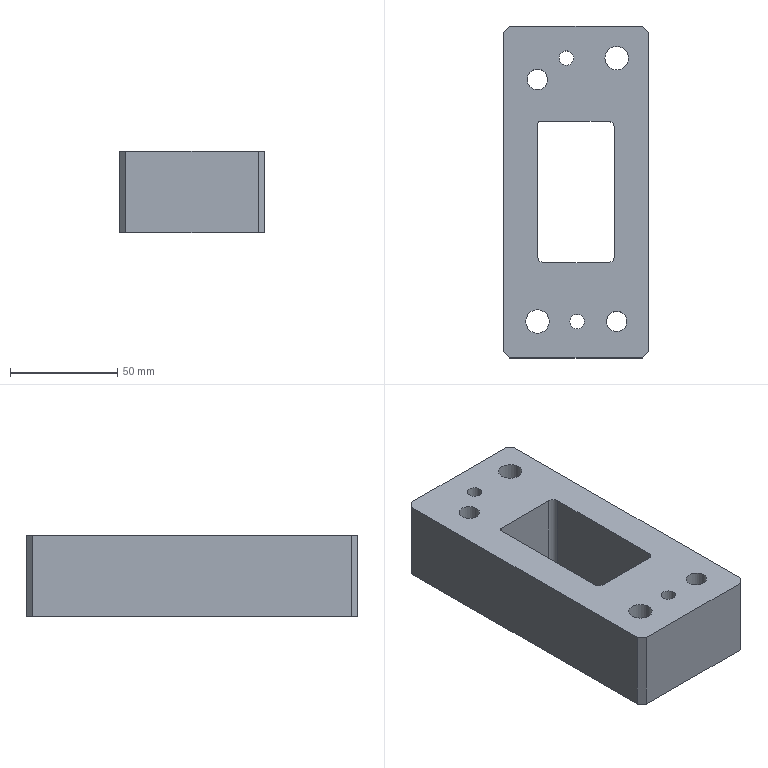Part | STEP file | 1_id174_x_t | 1 solid | 28 faces | box 68 x 155 x 38.1 mm | volume 290380 mm3 | plane 16 | cylinder 12 | commonest cylinder face diameters 6 x3 6.8 x2 9.525 x2 11 x2 18 x2 3 x1